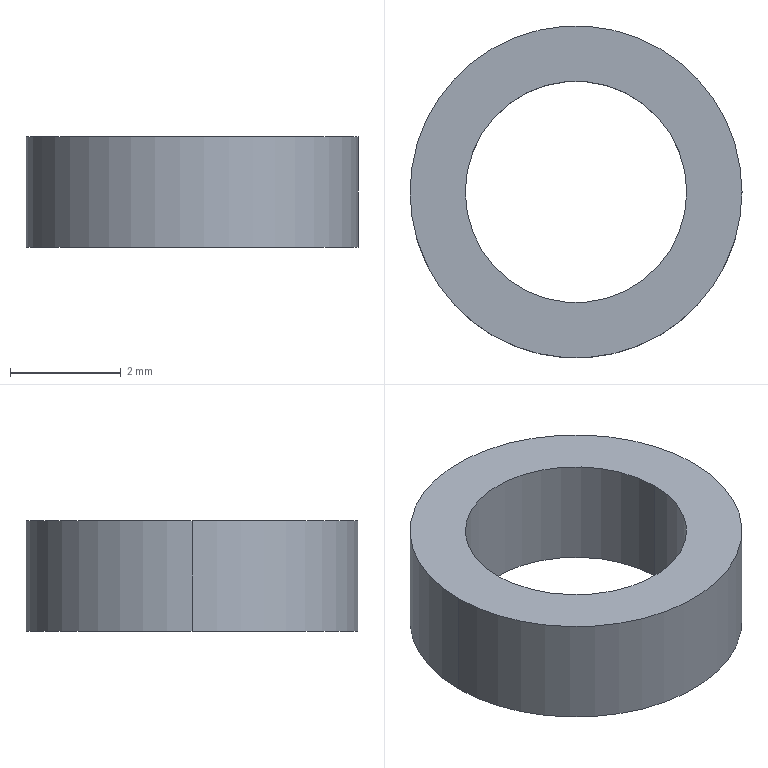Part | SolidWorks | features Extrusion 1 | 1 solid | 6 faces | box 6 x 6 x 2 mm | volume 31.416 mm3 | cylinder 4 | plane 2 | commonest cylinder face diameters 4 x2 6 x2
STEP:
#1=CARTESIAN_POINT('',(-2.,0.,2.));
#2=VERTEX_POINT('',#1);
#3=CARTESIAN_POINT('',(2.,0.,2.));
#4=VERTEX_POINT('',#3);
#5=CARTESIAN_POINT('',(0.,0.,2.));
#6=DIRECTION('',(0.,0.,1.));
#7=DIRECTION('',(1.,0.,0.));
#8=AXIS2_PLACEMENT_3D('',#5,#6,#7);
#9=CIRCLE('',#8,2.);
#10=EDGE_CURVE('',#2,#4,#9,.T.);
#11=ORIENTED_EDGE('',*,*,#10,.T.);
#12=CARTESIAN_POINT('',(2.,0.,0.));
#13=VERTEX_POINT('',#12);
#14=CARTESIAN_POINT('',(2.,0.,2.));
#15=DIRECTION('',(0.,0.,-1.));
#16=VECTOR('',#15,1000.);
#17=LINE('',#14,#16);
#18=EDGE_CURVE('',#4,#13,#17,.T.);
#19=ORIENTED_EDGE('',*,*,#18,.T.);
#20=CARTESIAN_POINT('',(-2.,0.,0.));
#21=VERTEX_POINT('',#20);
#22=CARTESIAN_POINT('',(0.,0.,0.));
#23=DIRECTION('',(0.,0.,1.));
#24=DIRECTION('',(1.,0.,0.));
#25=AXIS2_PLACEMENT_3D('',#22,#23,#24);
#26=CIRCLE('',#25,2.);
#27=EDGE_CURVE('',#21,#13,#26,.T.);
#28=ORIENTED_EDGE('',*,*,#27,.F.);
#29=CARTESIAN_POINT('',(-2.,0.,2.));
#30=DIRECTION('',(0.,0.,-1.));
#31=VECTOR('',#30,1000.);
#32=LINE('',#29,#31);
#33=EDGE_CURVE('',#2,#21,#32,.T.);
#34=ORIENTED_EDGE('',*,*,#33,.F.);
#35=EDGE_LOOP('',(#11,#19,#28,#34));
#36=FACE_OUTER_BOUND('',#35,.T.);
#37=CARTESIAN_POINT('',(0.,0.,2.));
#38=DIRECTION('',(0.,0.,-1.));
#39=DIRECTION('',(-1.,0.,0.));
#40=AXIS2_PLACEMENT_3D('',#37,#38,#39);
#41=CYLINDRICAL_SURFACE('',#40,2.);
#42=ADVANCED_FACE('',(#36),#41,.F.);
#43=CARTESIAN_POINT('',(3.,0.,2.));
#44=VERTEX_POINT('',#43);
#45=CARTESIAN_POINT('',(-3.,0.,2.));
#46=VERTEX_POINT('',#45);
#47=CARTESIAN_POINT('',(0.,0.,2.));
#48=DIRECTION('',(0.,0.,1.));
#49=DIRECTION('',(1.,0.,0.));
#50=AXIS2_PLACEMENT_3D('',#47,#48,#49);
#51=CIRCLE('',#50,3.);
#52=EDGE_CURVE('',#44,#46,#51,.T.);
#53=ORIENTED_EDGE('',*,*,#52,.F.);
#54=CARTESIAN_POINT('',(3.,0.,0.));
#55=VERTEX_POINT('',#54);
#56=CARTESIAN_POINT('',(3.,0.,2.));
#57=DIRECTION('',(0.,0.,-1.));
#58=VECTOR('',#57,1000.);
#59=LINE('',#56,#58);
#60=EDGE_CURVE('',#44,#55,#59,.T.);
#61=ORIENTED_EDGE('',*,*,#60,.T.);
#62=CARTESIAN_POINT('',(-3.,0.,0.));
#63=VERTEX_POINT('',#62);
#64=CARTESIAN_POINT('',(0.,0.,0.));
#65=DIRECTION('',(0.,0.,1.));
#66=DIRECTION('',(1.,0.,0.));
#67=AXIS2_PLACEMENT_3D('',#64,#65,#66);
#68=CIRCLE('',#67,3.);
#69=EDGE_CURVE('',#55,#63,#68,.T.);
#70=ORIENTED_EDGE('',*,*,#69,.T.);
#71=CARTESIAN_POINT('',(-3.,0.,2.));
#72=DIRECTION('',(0.,0.,-1.));
#73=VECTOR('',#72,1000.);
#74=LINE('',#71,#73);
#75=EDGE_CURVE('',#46,#63,#74,.T.);
#76=ORIENTED_EDGE('',*,*,#75,.F.);
#77=EDGE_LOOP('',(#53,#61,#70,#76));
#78=FACE_OUTER_BOUND('',#77,.T.);
#79=CARTESIAN_POINT('',(0.,0.,2.));
#80=DIRECTION('',(0.,0.,-1.));
#81=DIRECTION('',(-1.,0.,0.));
#82=AXIS2_PLACEMENT_3D('',#79,#80,#81);
#83=CYLINDRICAL_SURFACE('',#82,3.);
#84=ADVANCED_FACE('',(#78),#83,.T.);
#85=CARTESIAN_POINT('',(0.,0.,2.));
#86=DIRECTION('',(0.,0.,1.));
#87=DIRECTION('',(1.,0.,0.));
#88=AXIS2_PLACEMENT_3D('',#85,#86,#87);
#89=CIRCLE('',#88,3.);
#90=EDGE_CURVE('',#46,#44,#89,.T.);
#91=ORIENTED_EDGE('',*,*,#90,.T.);
#92=ORIENTED_EDGE('',*,*,#52,.T.);
#93=EDGE_LOOP('',(#91,#92));
#94=FACE_OUTER_BOUND('',#93,.T.);
#95=ORIENTED_EDGE('',*,*,#10,.F.);
#96=CARTESIAN_POINT('',(0.,0.,2.));
#97=DIRECTION('',(0.,0.,1.));
#98=DIRECTION('',(1.,0.,0.));
#99=AXIS2_PLACEMENT_3D('',#96,#97,#98);
#100=CIRCLE('',#99,2.);
#101=EDGE_CURVE('',#4,#2,#100,.T.);
#102=ORIENTED_EDGE('',*,*,#101,.F.);
#103=EDGE_LOOP('',(#95,#102));
#104=FACE_BOUND('',#103,.T.);
#105=CARTESIAN_POINT('',(0.,0.,2.));
#106=DIRECTION('',(0.,0.,1.));
#107=DIRECTION('',(1.,0.,0.));
#108=AXIS2_PLACEMENT_3D('',#105,#106,#107);
#109=PLANE('',#108);
#110=ADVANCED_FACE('',(#94,#104),#109,.T.);
#111=CARTESIAN_POINT('',(0.,0.,0.));
#112=DIRECTION('',(0.,0.,1.));
#113=DIRECTION('',(1.,0.,0.));
#114=AXIS2_PLACEMENT_3D('',#111,#112,#113);
#115=CIRCLE('',#114,3.);
#116=EDGE_CURVE('',#63,#55,#115,.T.);
#117=ORIENTED_EDGE('',*,*,#116,.F.);
#118=ORIENTED_EDGE('',*,*,#69,.F.);
#119=EDGE_LOOP('',(#117,#118));
#120=FACE_OUTER_BOUND('',#119,.T.);
#121=ORIENTED_EDGE('',*,*,#27,.T.);
#122=CARTESIAN_POINT('',(0.,0.,0.));
#123=DIRECTION('',(0.,0.,1.));
#124=DIRECTION('',(1.,0.,0.));
#125=AXIS2_PLACEMENT_3D('',#122,#123,#124);
#126=CIRCLE('',#125,2.);
#127=EDGE_CURVE('',#13,#21,#126,.T.);
#128=ORIENTED_EDGE('',*,*,#127,.T.);
#129=EDGE_LOOP('',(#121,#128));
#130=FACE_BOUND('',#129,.T.);
#131=CARTESIAN_POINT('',(0.,0.,0.));
#132=DIRECTION('',(0.,0.,1.));
#133=DIRECTION('',(1.,0.,0.));
#134=AXIS2_PLACEMENT_3D('',#131,#132,#133);
#135=PLANE('',#134);
#136=ADVANCED_FACE('',(#120,#130),#135,.F.);
#137=ORIENTED_EDGE('',*,*,#60,.F.);
#138=ORIENTED_EDGE('',*,*,#90,.F.);
#139=ORIENTED_EDGE('',*,*,#75,.T.);
#140=ORIENTED_EDGE('',*,*,#116,.T.);
#141=EDGE_LOOP('',(#137,#138,#139,#140));
#142=FACE_OUTER_BOUND('',#141,.T.);
#143=CARTESIAN_POINT('',(0.,0.,2.));
#144=DIRECTION('',(0.,0.,-1.));
#145=DIRECTION('',(-1.,0.,0.));
#146=AXIS2_PLACEMENT_3D('',#143,#144,#145);
#147=CYLINDRICAL_SURFACE('',#146,3.);
#148=ADVANCED_FACE('',(#142),#147,.T.);
#149=ORIENTED_EDGE('',*,*,#18,.F.);
#150=ORIENTED_EDGE('',*,*,#101,.T.);
#151=ORIENTED_EDGE('',*,*,#33,.T.);
#152=ORIENTED_EDGE('',*,*,#127,.F.);
#153=EDGE_LOOP('',(#149,#150,#151,#152));
#154=FACE_OUTER_BOUND('',#153,.T.);
#155=CARTESIAN_POINT('',(0.,0.,2.));
#156=DIRECTION('',(0.,0.,-1.));
#157=DIRECTION('',(-1.,0.,0.));
#158=AXIS2_PLACEMENT_3D('',#155,#156,#157);
#159=CYLINDRICAL_SURFACE('',#158,2.);
#160=ADVANCED_FACE('',(#154),#159,.F.);
#161=CLOSED_SHELL('',(#42,#84,#110,#136,#148,#160));
#162=MANIFOLD_SOLID_BREP('',#161);
#163=CARTESIAN_POINT('',(0.,0.,0.));
#164=DIRECTION('',(0.,0.,1.));
#165=DIRECTION('',(1.,0.,0.));
#166=AXIS2_PLACEMENT_3D('',#163,#164,#165);
#167=(LENGTH_UNIT()NAMED_UNIT(*)SI_UNIT(.MILLI.,.METRE.));
#168=UNCERTAINTY_MEASURE_WITH_UNIT(LENGTH_MEASURE(0.00001),#167,'','');
#169=(NAMED_UNIT(*)PLANE_ANGLE_UNIT()SI_UNIT($,.RADIAN.));
#170=(NAMED_UNIT(*)SI_UNIT($,.STERADIAN.)SOLID_ANGLE_UNIT());
#171=(GEOMETRIC_REPRESENTATION_CONTEXT(3)GLOBAL_UNCERTAINTY_ASSIGNED_CONTEXT((#168))GLOBAL_UNIT_ASSIGNED_CONTEXT((#167,#169,#170))REPRESENTATION_CONTEXT('',''));
#172=ADVANCED_BREP_SHAPE_REPRESENTATION('',(#162,#166),#171);